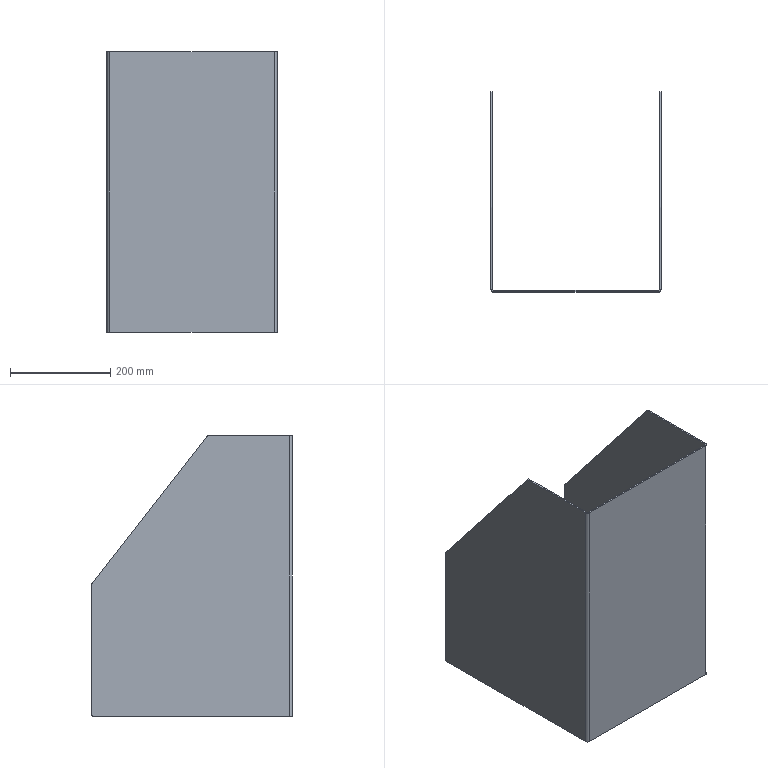Part | SolidWorks | features FlatPattern 1, ICE 1, SMBaseFlange 1, SheetMetal 1 | 1 solid | 30 faces | box 340 x 401 x 560 mm | volume 1696570 mm3 | plane 20 | cylinder 10 | commonest cylinder face diameters 6 x8 12 x2
STEP:
#1=CARTESIAN_POINT('',(340.,398.,0.));
#2=VERTEX_POINT('',#1);
#3=CARTESIAN_POINT('',(340.,401.,3.));
#4=VERTEX_POINT('',#3);
#5=CARTESIAN_POINT('',(340.,398.,3.));
#6=DIRECTION('',(1.,0.,0.));
#7=DIRECTION('',(0.,0.,1.));
#8=AXIS2_PLACEMENT_3D('',#5,#6,#7);
#9=CIRCLE('',#8,3.);
#10=EDGE_CURVE('',#2,#4,#9,.T.);
#11=ORIENTED_EDGE('',*,*,#10,.T.);
#12=CARTESIAN_POINT('',(340.,401.,262.937));
#13=VERTEX_POINT('',#12);
#14=CARTESIAN_POINT('',(340.,401.,560.));
#15=DIRECTION('',(0.,0.,-1.));
#16=VECTOR('',#15,1000.);
#17=LINE('',#14,#16);
#18=EDGE_CURVE('',#13,#4,#17,.T.);
#19=ORIENTED_EDGE('',*,*,#18,.F.);
#20=CARTESIAN_POINT('',(340.,400.364,264.784));
#21=VERTEX_POINT('',#20);
#22=CARTESIAN_POINT('',(340.,398.,262.937));
#23=DIRECTION('',(1.,0.,0.));
#24=DIRECTION('',(0.,0.,1.));
#25=AXIS2_PLACEMENT_3D('',#22,#23,#24);
#26=CIRCLE('',#25,3.);
#27=EDGE_CURVE('',#13,#21,#26,.T.);
#28=ORIENTED_EDGE('',*,*,#27,.T.);
#29=CARTESIAN_POINT('',(340.,170.611,558.847));
#30=VERTEX_POINT('',#29);
#31=CARTESIAN_POINT('',(340.,105.381,642.335));
#32=DIRECTION('',(0.,-0.6157,0.788));
#33=VECTOR('',#32,1000.);
#34=LINE('',#31,#33);
#35=EDGE_CURVE('',#21,#30,#34,.T.);
#36=ORIENTED_EDGE('',*,*,#35,.T.);
#37=CARTESIAN_POINT('',(340.,168.247,560.));
#38=VERTEX_POINT('',#37);
#39=CARTESIAN_POINT('',(340.,168.247,557.));
#40=DIRECTION('',(1.,0.,0.));
#41=DIRECTION('',(0.,0.,1.));
#42=AXIS2_PLACEMENT_3D('',#39,#40,#41);
#43=CIRCLE('',#42,3.);
#44=EDGE_CURVE('',#30,#38,#43,.T.);
#45=ORIENTED_EDGE('',*,*,#44,.T.);
#46=CARTESIAN_POINT('',(340.,6.,560.));
#47=VERTEX_POINT('',#46);
#48=CARTESIAN_POINT('',(340.,0.,560.));
#49=DIRECTION('',(0.,1.,0.));
#50=VECTOR('',#49,1000.);
#51=LINE('',#48,#50);
#52=EDGE_CURVE('',#47,#38,#51,.T.);
#53=ORIENTED_EDGE('',*,*,#52,.F.);
#54=CARTESIAN_POINT('',(340.,6.,0.));
#55=VERTEX_POINT('',#54);
#56=CARTESIAN_POINT('',(340.,6.,560.));
#57=DIRECTION('',(0.,0.,-1.));
#58=VECTOR('',#57,1000.);
#59=LINE('',#56,#58);
#60=EDGE_CURVE('',#47,#55,#59,.T.);
#61=ORIENTED_EDGE('',*,*,#60,.T.);
#62=CARTESIAN_POINT('',(340.,0.,0.));
#63=DIRECTION('',(0.,1.,0.));
#64=VECTOR('',#63,1000.);
#65=LINE('',#62,#64);
#66=EDGE_CURVE('',#55,#2,#65,.T.);
#67=ORIENTED_EDGE('',*,*,#66,.T.);
#68=EDGE_LOOP('',(#11,#19,#28,#36,#45,#53,#61,#67));
#69=FACE_OUTER_BOUND('',#68,.T.);
#70=CARTESIAN_POINT('',(340.,0.,560.));
#71=DIRECTION('',(-1.,0.,0.));
#72=DIRECTION('',(0.,0.,1.));
#73=AXIS2_PLACEMENT_3D('',#70,#71,#72);
#74=PLANE('',#73);
#75=ADVANCED_FACE('',(#69),#74,.F.);
#76=CARTESIAN_POINT('',(337.,401.,262.937));
#77=VERTEX_POINT('',#76);
#78=CARTESIAN_POINT('',(337.,401.,3.));
#79=VERTEX_POINT('',#78);
#80=CARTESIAN_POINT('',(337.,401.,560.));
#81=DIRECTION('',(0.,0.,-1.));
#82=VECTOR('',#81,1000.);
#83=LINE('',#80,#82);
#84=EDGE_CURVE('',#77,#79,#83,.T.);
#85=ORIENTED_EDGE('',*,*,#84,.T.);
#86=CARTESIAN_POINT('',(337.,398.,0.));
#87=VERTEX_POINT('',#86);
#88=CARTESIAN_POINT('',(337.,398.,3.));
#89=DIRECTION('',(1.,0.,0.));
#90=DIRECTION('',(0.,0.,1.));
#91=AXIS2_PLACEMENT_3D('',#88,#89,#90);
#92=CIRCLE('',#91,3.);
#93=EDGE_CURVE('',#87,#79,#92,.T.);
#94=ORIENTED_EDGE('',*,*,#93,.F.);
#95=CARTESIAN_POINT('',(337.,6.,0.));
#96=VERTEX_POINT('',#95);
#97=CARTESIAN_POINT('',(337.,0.,0.));
#98=DIRECTION('',(0.,1.,0.));
#99=VECTOR('',#98,1000.);
#100=LINE('',#97,#99);
#101=EDGE_CURVE('',#96,#87,#100,.T.);
#102=ORIENTED_EDGE('',*,*,#101,.F.);
#103=CARTESIAN_POINT('',(337.,6.,560.));
#104=VERTEX_POINT('',#103);
#105=CARTESIAN_POINT('',(337.,6.,560.));
#106=DIRECTION('',(0.,0.,-1.));
#107=VECTOR('',#106,1000.);
#108=LINE('',#105,#107);
#109=EDGE_CURVE('',#104,#96,#108,.T.);
#110=ORIENTED_EDGE('',*,*,#109,.F.);
#111=CARTESIAN_POINT('',(337.,168.247,560.));
#112=VERTEX_POINT('',#111);
#113=CARTESIAN_POINT('',(337.,0.,560.));
#114=DIRECTION('',(0.,1.,0.));
#115=VECTOR('',#114,1000.);
#116=LINE('',#113,#115);
#117=EDGE_CURVE('',#104,#112,#116,.T.);
#118=ORIENTED_EDGE('',*,*,#117,.T.);
#119=CARTESIAN_POINT('',(337.,170.611,558.847));
#120=VERTEX_POINT('',#119);
#121=CARTESIAN_POINT('',(337.,168.247,557.));
#122=DIRECTION('',(1.,0.,0.));
#123=DIRECTION('',(0.,0.,1.));
#124=AXIS2_PLACEMENT_3D('',#121,#122,#123);
#125=CIRCLE('',#124,3.);
#126=EDGE_CURVE('',#120,#112,#125,.T.);
#127=ORIENTED_EDGE('',*,*,#126,.F.);
#128=CARTESIAN_POINT('',(337.,400.364,264.784));
#129=VERTEX_POINT('',#128);
#130=CARTESIAN_POINT('',(337.,105.381,642.335));
#131=DIRECTION('',(0.,-0.6157,0.788));
#132=VECTOR('',#131,1000.);
#133=LINE('',#130,#132);
#134=EDGE_CURVE('',#129,#120,#133,.T.);
#135=ORIENTED_EDGE('',*,*,#134,.F.);
#136=CARTESIAN_POINT('',(337.,398.,262.937));
#137=DIRECTION('',(1.,0.,0.));
#138=DIRECTION('',(0.,0.,1.));
#139=AXIS2_PLACEMENT_3D('',#136,#137,#138);
#140=CIRCLE('',#139,3.);
#141=EDGE_CURVE('',#77,#129,#140,.T.);
#142=ORIENTED_EDGE('',*,*,#141,.F.);
#143=EDGE_LOOP('',(#85,#94,#102,#110,#118,#127,#135,#142));
#144=FACE_OUTER_BOUND('',#143,.T.);
#145=CARTESIAN_POINT('',(337.,0.,560.));
#146=DIRECTION('',(-1.,0.,0.));
#147=DIRECTION('',(0.,0.,1.));
#148=AXIS2_PLACEMENT_3D('',#145,#146,#147);
#149=PLANE('',#148);
#150=ADVANCED_FACE('',(#144),#149,.T.);
#151=ORIENTED_EDGE('',*,*,#18,.T.);
#152=CARTESIAN_POINT('',(337.,401.,3.));
#153=DIRECTION('',(1.,0.,0.));
#154=VECTOR('',#153,1000.);
#155=LINE('',#152,#154);
#156=EDGE_CURVE('',#79,#4,#155,.T.);
#157=ORIENTED_EDGE('',*,*,#156,.F.);
#158=ORIENTED_EDGE('',*,*,#84,.F.);
#159=CARTESIAN_POINT('',(337.,401.,262.937));
#160=DIRECTION('',(1.,0.,0.));
#161=VECTOR('',#160,1000.);
#162=LINE('',#159,#161);
#163=EDGE_CURVE('',#77,#13,#162,.T.);
#164=ORIENTED_EDGE('',*,*,#163,.T.);
#165=EDGE_LOOP('',(#151,#157,#158,#164));
#166=FACE_OUTER_BOUND('',#165,.T.);
#167=CARTESIAN_POINT('',(337.,401.,560.));
#168=DIRECTION('',(0.,1.,0.));
#169=DIRECTION('',(0.,0.,1.));
#170=AXIS2_PLACEMENT_3D('',#167,#168,#169);
#171=PLANE('',#170);
#172=ADVANCED_FACE('',(#166),#171,.T.);
#173=CARTESIAN_POINT('',(3.,398.,0.));
#174=VERTEX_POINT('',#173);
#175=CARTESIAN_POINT('',(3.,6.,0.));
#176=VERTEX_POINT('',#175);
#177=CARTESIAN_POINT('',(3.,0.,0.));
#178=DIRECTION('',(0.,-1.,0.));
#179=VECTOR('',#178,1000.);
#180=LINE('',#177,#179);
#181=EDGE_CURVE('',#174,#176,#180,.T.);
#182=ORIENTED_EDGE('',*,*,#181,.F.);
#183=CARTESIAN_POINT('',(3.,401.,3.));
#184=VERTEX_POINT('',#183);
#185=CARTESIAN_POINT('',(3.,398.,3.));
#186=DIRECTION('',(-1.,0.,0.));
#187=DIRECTION('',(0.,0.,-1.));
#188=AXIS2_PLACEMENT_3D('',#185,#186,#187);
#189=CIRCLE('',#188,3.);
#190=EDGE_CURVE('',#184,#174,#189,.T.);
#191=ORIENTED_EDGE('',*,*,#190,.F.);
#192=CARTESIAN_POINT('',(3.,401.,262.937));
#193=VERTEX_POINT('',#192);
#194=CARTESIAN_POINT('',(3.,401.,560.));
#195=DIRECTION('',(0.,0.,-1.));
#196=VECTOR('',#195,1000.);
#197=LINE('',#194,#196);
#198=EDGE_CURVE('',#193,#184,#197,.T.);
#199=ORIENTED_EDGE('',*,*,#198,.F.);
#200=CARTESIAN_POINT('',(3.,400.364,264.784));
#201=VERTEX_POINT('',#200);
#202=CARTESIAN_POINT('',(3.,398.,262.937));
#203=DIRECTION('',(-1.,0.,0.));
#204=DIRECTION('',(0.,0.,-1.));
#205=AXIS2_PLACEMENT_3D('',#202,#203,#204);
#206=CIRCLE('',#205,3.);
#207=EDGE_CURVE('',#201,#193,#206,.T.);
#208=ORIENTED_EDGE('',*,*,#207,.F.);
#209=CARTESIAN_POINT('',(3.,170.611,558.847));
#210=VERTEX_POINT('',#209);
#211=CARTESIAN_POINT('',(3.,105.381,642.335));
#212=DIRECTION('',(0.,0.6157,-0.788));
#213=VECTOR('',#212,1000.);
#214=LINE('',#211,#213);
#215=EDGE_CURVE('',#210,#201,#214,.T.);
#216=ORIENTED_EDGE('',*,*,#215,.F.);
#217=CARTESIAN_POINT('',(3.,168.247,560.));
#218=VERTEX_POINT('',#217);
#219=CARTESIAN_POINT('',(3.,168.247,557.));
#220=DIRECTION('',(-1.,0.,0.));
#221=DIRECTION('',(0.,0.,-1.));
#222=AXIS2_PLACEMENT_3D('',#219,#220,#221);
#223=CIRCLE('',#222,3.);
#224=EDGE_CURVE('',#218,#210,#223,.T.);
#225=ORIENTED_EDGE('',*,*,#224,.F.);
#226=CARTESIAN_POINT('',(3.,6.,560.));
#227=VERTEX_POINT('',#226);
#228=CARTESIAN_POINT('',(3.,0.,560.));
#229=DIRECTION('',(0.,-1.,0.));
#230=VECTOR('',#229,1000.);
#231=LINE('',#228,#230);
#232=EDGE_CURVE('',#218,#227,#231,.T.);
#233=ORIENTED_EDGE('',*,*,#232,.T.);
#234=CARTESIAN_POINT('',(3.,6.,560.));
#235=DIRECTION('',(0.,0.,-1.));
#236=VECTOR('',#235,1000.);
#237=LINE('',#234,#236);
#238=EDGE_CURVE('',#227,#176,#237,.T.);
#239=ORIENTED_EDGE('',*,*,#238,.T.);
#240=EDGE_LOOP('',(#182,#191,#199,#208,#216,#225,#233,#239));
#241=FACE_OUTER_BOUND('',#240,.T.);
#242=CARTESIAN_POINT('',(3.,0.,560.));
#243=DIRECTION('',(1.,0.,0.));
#244=DIRECTION('',(0.,0.,-1.));
#245=AXIS2_PLACEMENT_3D('',#242,#243,#244);
#246=PLANE('',#245);
#247=ADVANCED_FACE('',(#241),#246,.T.);
#248=CARTESIAN_POINT('',(0.,401.,3.));
#249=VERTEX_POINT('',#248);
#250=CARTESIAN_POINT('',(0.,398.,0.));
#251=VERTEX_POINT('',#250);
#252=CARTESIAN_POINT('',(0.,398.,3.));
#253=DIRECTION('',(-1.,0.,0.));
#254=DIRECTION('',(0.,0.,-1.));
#255=AXIS2_PLACEMENT_3D('',#252,#253,#254);
#256=CIRCLE('',#255,3.);
#257=EDGE_CURVE('',#249,#251,#256,.T.);
#258=ORIENTED_EDGE('',*,*,#257,.T.);
#259=CARTESIAN_POINT('',(0.,6.,0.));
#260=VERTEX_POINT('',#259);
#261=CARTESIAN_POINT('',(0.,0.,0.));
#262=DIRECTION('',(0.,-1.,0.));
#263=VECTOR('',#262,1000.);
#264=LINE('',#261,#263);
#265=EDGE_CURVE('',#251,#260,#264,.T.);
#266=ORIENTED_EDGE('',*,*,#265,.T.);
#267=CARTESIAN_POINT('',(0.,6.,560.));
#268=VERTEX_POINT('',#267);
#269=CARTESIAN_POINT('',(0.,6.,560.));
#270=DIRECTION('',(0.,0.,-1.));
#271=VECTOR('',#270,1000.);
#272=LINE('',#269,#271);
#273=EDGE_CURVE('',#268,#260,#272,.T.);
#274=ORIENTED_EDGE('',*,*,#273,.F.);
#275=CARTESIAN_POINT('',(0.,168.247,560.));
#276=VERTEX_POINT('',#275);
#277=CARTESIAN_POINT('',(0.,0.,560.));
#278=DIRECTION('',(0.,-1.,0.));
#279=VECTOR('',#278,1000.);
#280=LINE('',#277,#279);
#281=EDGE_CURVE('',#276,#268,#280,.T.);
#282=ORIENTED_EDGE('',*,*,#281,.F.);
#283=CARTESIAN_POINT('',(0.,170.611,558.847));
#284=VERTEX_POINT('',#283);
#285=CARTESIAN_POINT('',(0.,168.247,557.));
#286=DIRECTION('',(-1.,0.,0.));
#287=DIRECTION('',(0.,0.,-1.));
#288=AXIS2_PLACEMENT_3D('',#285,#286,#287);
#289=CIRCLE('',#288,3.);
#290=EDGE_CURVE('',#276,#284,#289,.T.);
#291=ORIENTED_EDGE('',*,*,#290,.T.);
#292=CARTESIAN_POINT('',(0.,400.364,264.784));
#293=VERTEX_POINT('',#292);
#294=CARTESIAN_POINT('',(0.,105.381,642.335));
#295=DIRECTION('',(0.,0.6157,-0.788));
#296=VECTOR('',#295,1000.);
#297=LINE('',#294,#296);
#298=EDGE_CURVE('',#284,#293,#297,.T.);
#299=ORIENTED_EDGE('',*,*,#298,.T.);
#300=CARTESIAN_POINT('',(0.,401.,262.937));
#301=VERTEX_POINT('',#300);
#302=CARTESIAN_POINT('',(0.,398.,262.937));
#303=DIRECTION('',(-1.,0.,0.));
#304=DIRECTION('',(0.,0.,-1.));
#305=AXIS2_PLACEMENT_3D('',#302,#303,#304);
#306=CIRCLE('',#305,3.);
#307=EDGE_CURVE('',#293,#301,#306,.T.);
#308=ORIENTED_EDGE('',*,*,#307,.T.);
#309=CARTESIAN_POINT('',(0.,401.,560.));
#310=DIRECTION('',(0.,0.,-1.));
#311=VECTOR('',#310,1000.);
#312=LINE('',#309,#311);
#313=EDGE_CURVE('',#301,#249,#312,.T.);
#314=ORIENTED_EDGE('',*,*,#313,.T.);
#315=EDGE_LOOP('',(#258,#266,#274,#282,#291,#299,#308,#314));
#316=FACE_OUTER_BOUND('',#315,.T.);
#317=CARTESIAN_POINT('',(0.,0.,560.));
#318=DIRECTION('',(1.,0.,0.));
#319=DIRECTION('',(0.,0.,-1.));
#320=AXIS2_PLACEMENT_3D('',#317,#318,#319);
#321=PLANE('',#320);
#322=ADVANCED_FACE('',(#316),#321,.F.);
#323=ORIENTED_EDGE('',*,*,#52,.T.);
#324=CARTESIAN_POINT('',(337.,168.247,560.));
#325=DIRECTION('',(1.,0.,0.));
#326=VECTOR('',#325,1000.);
#327=LINE('',#324,#326);
#328=EDGE_CURVE('',#112,#38,#327,.T.);
#329=ORIENTED_EDGE('',*,*,#328,.F.);
#330=ORIENTED_EDGE('',*,*,#117,.F.);
#331=CARTESIAN_POINT('',(337.,6.,560.));
#332=DIRECTION('',(1.,0.,0.));
#333=VECTOR('',#332,1000.);
#334=LINE('',#331,#333);
#335=EDGE_CURVE('',#104,#47,#334,.T.);
#336=ORIENTED_EDGE('',*,*,#335,.T.);
#337=EDGE_LOOP('',(#323,#329,#330,#336));
#338=FACE_OUTER_BOUND('',#337,.T.);
#339=CARTESIAN_POINT('',(334.,6.,560.));
#340=DIRECTION('',(0.,0.,1.));
#341=DIRECTION('',(1.,0.,0.));
#342=AXIS2_PLACEMENT_3D('',#339,#340,#341);
#343=PLANE('',#342);
#344=ADVANCED_FACE('',(#338),#343,.T.);
#345=CARTESIAN_POINT('',(3.,401.,3.));
#346=DIRECTION('',(-1.,0.,0.));
#347=VECTOR('',#346,1000.);
#348=LINE('',#345,#347);
#349=EDGE_CURVE('',#184,#249,#348,.T.);
#350=ORIENTED_EDGE('',*,*,#349,.T.);
#351=ORIENTED_EDGE('',*,*,#313,.F.);
#352=CARTESIAN_POINT('',(3.,401.,262.937));
#353=DIRECTION('',(-1.,0.,0.));
#354=VECTOR('',#353,1000.);
#355=LINE('',#352,#354);
#356=EDGE_CURVE('',#193,#301,#355,.T.);
#357=ORIENTED_EDGE('',*,*,#356,.F.);
#358=ORIENTED_EDGE('',*,*,#198,.T.);
#359=EDGE_LOOP('',(#350,#351,#357,#358));
#360=FACE_OUTER_BOUND('',#359,.T.);
#361=CARTESIAN_POINT('',(0.,401.,560.));
#362=DIRECTION('',(0.,1.,0.));
#363=DIRECTION('',(0.,0.,1.));
#364=AXIS2_PLACEMENT_3D('',#361,#362,#363);
#365=PLANE('',#364);
#366=ADVANCED_FACE('',(#360),#365,.T.);
#367=CARTESIAN_POINT('',(0.,6.,560.));
#368=DIRECTION('',(1.,0.,0.));
#369=VECTOR('',#368,1000.);
#370=LINE('',#367,#369);
#371=EDGE_CURVE('',#268,#227,#370,.T.);
#372=ORIENTED_EDGE('',*,*,#371,.F.);
#373=CARTESIAN_POINT('',(6.,0.,560.));
#374=VERTEX_POINT('',#373);
#375=CARTESIAN_POINT('',(6.,6.,560.));
#376=DIRECTION('',(0.,0.,1.));
#377=DIRECTION('',(-1.,0.,0.));
#378=AXIS2_PLACEMENT_3D('',#375,#376,#377);
#379=CIRCLE('',#378,6.);
#380=EDGE_CURVE('',#268,#374,#379,.T.);
#381=ORIENTED_EDGE('',*,*,#380,.T.);
#382=CARTESIAN_POINT('',(6.,3.,560.));
#383=VERTEX_POINT('',#382);
#384=CARTESIAN_POINT('',(6.,3.,560.));
#385=DIRECTION('',(0.,-1.,0.));
#386=VECTOR('',#385,1000.);
#387=LINE('',#384,#386);
#388=EDGE_CURVE('',#383,#374,#387,.T.);
#389=ORIENTED_EDGE('',*,*,#388,.F.);
#390=CARTESIAN_POINT('',(6.,6.,560.));
#391=DIRECTION('',(0.,0.,1.));
#392=DIRECTION('',(1.,0.,0.));
#393=AXIS2_PLACEMENT_3D('',#390,#391,#392);
#394=CIRCLE('',#393,3.);
#395=EDGE_CURVE('',#227,#383,#394,.T.);
#396=ORIENTED_EDGE('',*,*,#395,.F.);
#397=EDGE_LOOP('',(#372,#381,#389,#396));
#398=FACE_OUTER_BOUND('',#397,.T.);
#399=CARTESIAN_POINT('',(0.,6.,560.));
#400=DIRECTION('',(0.,0.,1.));
#401=DIRECTION('',(1.,0.,0.));
#402=AXIS2_PLACEMENT_3D('',#399,#400,#401);
#403=PLANE('',#402);
#404=ADVANCED_FACE('',(#398),#403,.T.);
#405=CARTESIAN_POINT('',(3.,168.247,560.));
#406=DIRECTION('',(-1.,0.,0.));
#407=VECTOR('',#406,1000.);
#408=LINE('',#405,#407);
#409=EDGE_CURVE('',#218,#276,#408,.T.);
#410=ORIENTED_EDGE('',*,*,#409,.T.);
#411=ORIENTED_EDGE('',*,*,#281,.T.);
#412=ORIENTED_EDGE('',*,*,#371,.T.);
#413=ORIENTED_EDGE('',*,*,#232,.F.);
#414=EDGE_LOOP('',(#410,#411,#412,#413));
#415=FACE_OUTER_BOUND('',#414,.T.);
#416=CARTESIAN_POINT('',(6.,3.,560.));
#417=DIRECTION('',(0.,0.,1.));
#418=DIRECTION('',(1.,0.,0.));
#419=AXIS2_PLACEMENT_3D('',#416,#417,#418);
#420=PLANE('',#419);
#421=ADVANCED_FACE('',(#415),#420,.T.);
#422=CARTESIAN_POINT('',(6.,0.,0.));
#423=VERTEX_POINT('',#422);
#424=CARTESIAN_POINT('',(6.,3.,0.));
#425=VERTEX_POINT('',#424);
#426=CARTESIAN_POINT('',(6.,0.,0.));
#427=DIRECTION('',(0.,1.,0.));
#428=VECTOR('',#427,1000.);
#429=LINE('',#426,#428);
#430=EDGE_CURVE('',#423,#425,#429,.T.);
#431=ORIENTED_EDGE('',*,*,#430,.F.);
#432=CARTESIAN_POINT('',(6.,6.,0.));
#433=DIRECTION('',(0.,0.,1.));
#434=DIRECTION('',(-1.,0.,0.));
#435=AXIS2_PLACEMENT_3D('',#432,#433,#434);
#436=CIRCLE('',#435,6.);
#437=EDGE_CURVE('',#260,#423,#436,.T.);
#438=ORIENTED_EDGE('',*,*,#437,.F.);
#439=CARTESIAN_POINT('',(3.,6.,0.));
#440=DIRECTION('',(-1.,0.,0.));
#441=VECTOR('',#440,1000.);
#442=LINE('',#439,#441);
#443=EDGE_CURVE('',#176,#260,#442,.T.);
#444=ORIENTED_EDGE('',*,*,#443,.F.);
#445=CARTESIAN_POINT('',(6.,6.,0.));
#446=DIRECTION('',(0.,0.,1.));
#447=DIRECTION('',(1.,0.,0.));
#448=AXIS2_PLACEMENT_3D('',#445,#446,#447);
#449=CIRCLE('',#448,3.);
#450=EDGE_CURVE('',#176,#425,#449,.T.);
#451=ORIENTED_EDGE('',*,*,#450,.T.);
#452=EDGE_LOOP('',(#431,#438,#444,#451));
#453=FACE_OUTER_BOUND('',#452,.T.);
#454=CARTESIAN_POINT('',(6.,0.,0.));
#455=DIRECTION('',(0.,0.,-1.));
#456=DIRECTION('',(-1.,0.,0.));
#457=AXIS2_PLACEMENT_3D('',#454,#455,#456);
#458=PLANE('',#457);
#459=ADVANCED_FACE('',(#453),#458,.T.);
#460=CARTESIAN_POINT('',(334.,0.,0.));
#461=VERTEX_POINT('',#460);
#462=CARTESIAN_POINT('',(0.,0.,0.));
#463=DIRECTION('',(1.,0.,0.));
#464=VECTOR('',#463,1000.);
#465=LINE('',#462,#464);
#466=EDGE_CURVE('',#423,#461,#465,.T.);
#467=ORIENTED_EDGE('',*,*,#466,.F.);
#468=ORIENTED_EDGE('',*,*,#430,.T.);
#469=CARTESIAN_POINT('',(334.,3.,0.));
#470=VERTEX_POINT('',#469);
#471=CARTESIAN_POINT('',(0.,3.,0.));
#472=DIRECTION('',(1.,0.,0.));
#473=VECTOR('',#472,1000.);
#474=LINE('',#471,#473);
#475=EDGE_CURVE('',#425,#470,#474,.T.);
#476=ORIENTED_EDGE('',*,*,#475,.T.);
#477=CARTESIAN_POINT('',(334.,3.,0.));
#478=DIRECTION('',(0.,-1.,0.));
#479=VECTOR('',#478,1000.);
#480=LINE('',#477,#479);
#481=EDGE_CURVE('',#470,#461,#480,.T.);
#482=ORIENTED_EDGE('',*,*,#481,.T.);
#483=EDGE_LOOP('',(#467,#468,#476,#482));
#484=FACE_OUTER_BOUND('',#483,.T.);
#485=CARTESIAN_POINT('',(3.,6.,0.));
#486=DIRECTION('',(0.,0.,-1.));
#487=DIRECTION('',(-1.,0.,0.));
#488=AXIS2_PLACEMENT_3D('',#485,#486,#487);
#489=PLANE('',#488);
#490=ADVANCED_FACE('',(#484),#489,.T.);
#491=CARTESIAN_POINT('',(334.,0.,560.));
#492=VERTEX_POINT('',#491);
#493=CARTESIAN_POINT('',(334.,3.,560.));
#494=VERTEX_POINT('',#493);
#495=CARTESIAN_POINT('',(334.,0.,560.));
#496=DIRECTION('',(0.,1.,0.));
#497=VECTOR('',#496,1000.);
#498=LINE('',#495,#497);
#499=EDGE_CURVE('',#492,#494,#498,.T.);
#500=ORIENTED_EDGE('',*,*,#499,.F.);
#501=CARTESIAN_POINT('',(334.,6.,560.));
#502=DIRECTION('',(0.,0.,1.));
#503=DIRECTION('',(-1.,0.,0.));
#504=AXIS2_PLACEMENT_3D('',#501,#502,#503);
#505=CIRCLE('',#504,6.);
#506=EDGE_CURVE('',#492,#47,#505,.T.);
#507=ORIENTED_EDGE('',*,*,#506,.T.);
#508=ORIENTED_EDGE('',*,*,#335,.F.);
#509=CARTESIAN_POINT('',(334.,6.,560.));
#510=DIRECTION('',(0.,0.,1.));
#511=DIRECTION('',(1.,0.,0.));
#512=AXIS2_PLACEMENT_3D('',#509,#510,#511);
#513=CIRCLE('',#512,3.);
#514=EDGE_CURVE('',#494,#104,#513,.T.);
#515=ORIENTED_EDGE('',*,*,#514,.F.);
#516=EDGE_LOOP('',(#500,#507,#508,#515));
#517=FACE_OUTER_BOUND('',#516,.T.);
#518=CARTESIAN_POINT('',(334.,0.,560.));
#519=DIRECTION('',(0.,0.,1.));
#520=DIRECTION('',(1.,0.,0.));
#521=AXIS2_PLACEMENT_3D('',#518,#519,#520);
#522=PLANE('',#521);
#523=ADVANCED_FACE('',(#517),#522,.T.);
#524=CARTESIAN_POINT('',(0.,0.,560.));
#525=DIRECTION('',(1.,0.,0.));
#526=VECTOR('',#525,1000.);
#527=LINE('',#524,#526);
#528=EDGE_CURVE('',#374,#492,#527,.T.);
#529=ORIENTED_EDGE('',*,*,#528,.T.);
#530=ORIENTED_EDGE('',*,*,#499,.T.);
#531=CARTESIAN_POINT('',(0.,3.,560.));
#532=DIRECTION('',(1.,0.,0.));
#533=VECTOR('',#532,1000.);
#534=LINE('',#531,#533);
#535=EDGE_CURVE('',#383,#494,#534,.T.);
#536=ORIENTED_EDGE('',*,*,#535,.F.);
#537=ORIENTED_EDGE('',*,*,#388,.T.);
#538=EDGE_LOOP('',(#529,#530,#536,#537));
#539=FACE_OUTER_BOUND('',#538,.T.);
#540=CARTESIAN_POINT('',(337.,6.,560.));
#541=DIRECTION('',(0.,0.,1.));
#542=DIRECTION('',(1.,0.,0.));
#543=AXIS2_PLACEMENT_3D('',#540,#541,#542);
#544=PLANE('',#543);
#545=ADVANCED_FACE('',(#539),#544,.T.);
#546=CARTESIAN_POINT('',(340.,6.,0.));
#547=DIRECTION('',(-1.,0.,0.));
#548=VECTOR('',#547,1000.);
#549=LINE('',#546,#548);
#550=EDGE_CURVE('',#55,#96,#549,.T.);
#551=ORIENTED_EDGE('',*,*,#550,.F.);
#552=CARTESIAN_POINT('',(334.,6.,0.));
#553=DIRECTION('',(0.,0.,1.));
#554=DIRECTION('',(-1.,0.,0.));
#555=AXIS2_PLACEMENT_3D('',#552,#553,#554);
#556=CIRCLE('',#555,6.);
#557=EDGE_CURVE('',#461,#55,#556,.T.);
#558=ORIENTED_EDGE('',*,*,#557,.F.);
#559=ORIENTED_EDGE('',*,*,#481,.F.);
#560=CARTESIAN_POINT('',(334.,6.,0.));
#561=DIRECTION('',(0.,0.,1.));
#562=DIRECTION('',(1.,0.,0.));
#563=AXIS2_PLACEMENT_3D('',#560,#561,#562);
#564=CIRCLE('',#563,3.);
#565=EDGE_CURVE('',#470,#96,#564,.T.);
#566=ORIENTED_EDGE('',*,*,#565,.T.);
#567=EDGE_LOOP('',(#551,#558,#559,#566));
#568=FACE_OUTER_BOUND('',#567,.T.);
#569=CARTESIAN_POINT('',(340.,6.,0.));
#570=DIRECTION('',(0.,0.,-1.));
#571=DIRECTION('',(-1.,0.,0.));
#572=AXIS2_PLACEMENT_3D('',#569,#570,#571);
#573=PLANE('',#572);
#574=ADVANCED_FACE('',(#568),#573,.T.);
#575=CARTESIAN_POINT('',(337.,398.,0.));
#576=DIRECTION('',(1.,0.,0.));
#577=VECTOR('',#576,1000.);
#578=LINE('',#575,#577);
#579=EDGE_CURVE('',#87,#2,#578,.T.);
#580=ORIENTED_EDGE('',*,*,#579,.T.);
#581=ORIENTED_EDGE('',*,*,#66,.F.);
#582=ORIENTED_EDGE('',*,*,#550,.T.);
#583=ORIENTED_EDGE('',*,*,#101,.T.);
#584=EDGE_LOOP('',(#580,#581,#582,#583));
#585=FACE_OUTER_BOUND('',#584,.T.);
#586=CARTESIAN_POINT('',(334.,3.,0.));
#587=DIRECTION('',(0.,0.,-1.));
#588=DIRECTION('',(-1.,0.,0.));
#589=AXIS2_PLACEMENT_3D('',#586,#587,#588);
#590=PLANE('',#589);
#591=ADVANCED_FACE('',(#585),#590,.T.);
#592=ORIENTED_EDGE('',*,*,#565,.F.);
#593=CARTESIAN_POINT('',(334.,3.,560.));
#594=DIRECTION('',(0.,0.,-1.));
#595=VECTOR('',#594,1000.);
#596=LINE('',#593,#595);
#597=EDGE_CURVE('',#494,#470,#596,.T.);
#598=ORIENTED_EDGE('',*,*,#597,.F.);
#599=ORIENTED_EDGE('',*,*,#514,.T.);
#600=ORIENTED_EDGE('',*,*,#109,.T.);
#601=EDGE_LOOP('',(#592,#598,#599,#600));
#602=FACE_OUTER_BOUND('',#601,.T.);
#603=CARTESIAN_POINT('',(334.,6.,560.));
#604=DIRECTION('',(0.,0.,-1.));
#605=DIRECTION('',(-1.,0.,0.));
#606=AXIS2_PLACEMENT_3D('',#603,#604,#605);
#607=CYLINDRICAL_SURFACE('',#606,3.);
#608=ADVANCED_FACE('',(#602),#607,.F.);
#609=ORIENTED_EDGE('',*,*,#475,.F.);
#610=CARTESIAN_POINT('',(6.,3.,560.));
#611=DIRECTION('',(0.,0.,-1.));
#612=VECTOR('',#611,1000.);
#613=LINE('',#610,#612);
#614=EDGE_CURVE('',#383,#425,#613,.T.);
#615=ORIENTED_EDGE('',*,*,#614,.F.);
#616=ORIENTED_EDGE('',*,*,#535,.T.);
#617=ORIENTED_EDGE('',*,*,#597,.T.);
#618=EDGE_LOOP('',(#609,#615,#616,#617));
#619=FACE_OUTER_BOUND('',#618,.T.);
#620=CARTESIAN_POINT('',(0.,3.,560.));
#621=DIRECTION('',(0.,1.,0.));
#622=DIRECTION('',(0.,0.,1.));
#623=AXIS2_PLACEMENT_3D('',#620,#621,#622);
#624=PLANE('',#623);
#625=ADVANCED_FACE('',(#619),#624,.T.);
#626=ORIENTED_EDGE('',*,*,#450,.F.);
#627=ORIENTED_EDGE('',*,*,#238,.F.);
#628=ORIENTED_EDGE('',*,*,#395,.T.);
#629=ORIENTED_EDGE('',*,*,#614,.T.);
#630=EDGE_LOOP('',(#626,#627,#628,#629));
#631=FACE_OUTER_BOUND('',#630,.T.);
#632=CARTESIAN_POINT('',(6.,6.,560.));
#633=DIRECTION('',(0.,0.,-1.));
#634=DIRECTION('',(-1.,0.,0.));
#635=AXIS2_PLACEMENT_3D('',#632,#633,#634);
#636=CYLINDRICAL_SURFACE('',#635,3.);
#637=ADVANCED_FACE('',(#631),#636,.F.);
#638=ORIENTED_EDGE('',*,*,#437,.T.);
#639=CARTESIAN_POINT('',(6.,0.,560.));
#640=DIRECTION('',(0.,0.,-1.));
#641=VECTOR('',#640,1000.);
#642=LINE('',#639,#641);
#643=EDGE_CURVE('',#374,#423,#642,.T.);
#644=ORIENTED_EDGE('',*,*,#643,.F.);
#645=ORIENTED_EDGE('',*,*,#380,.F.);
#646=ORIENTED_EDGE('',*,*,#273,.T.);
#647=EDGE_LOOP('',(#638,#644,#645,#646));
#648=FACE_OUTER_BOUND('',#647,.T.);
#649=CARTESIAN_POINT('',(6.,6.,560.));
#650=DIRECTION('',(0.,0.,-1.));
#651=DIRECTION('',(-1.,0.,0.));
#652=AXIS2_PLACEMENT_3D('',#649,#650,#651);
#653=CYLINDRICAL_SURFACE('',#652,6.);
#654=ADVANCED_FACE('',(#648),#653,.T.);
#655=ORIENTED_EDGE('',*,*,#466,.T.);
#656=CARTESIAN_POINT('',(334.,0.,560.));
#657=DIRECTION('',(0.,0.,-1.));
#658=VECTOR('',#657,1000.);
#659=LINE('',#656,#658);
#660=EDGE_CURVE('',#492,#461,#659,.T.);
#661=ORIENTED_EDGE('',*,*,#660,.F.);
#662=ORIENTED_EDGE('',*,*,#528,.F.);
#663=ORIENTED_EDGE('',*,*,#643,.T.);
#664=EDGE_LOOP('',(#655,#661,#662,#663));
#665=FACE_OUTER_BOUND('',#664,.T.);
#666=CARTESIAN_POINT('',(0.,0.,560.));
#667=DIRECTION('',(0.,1.,0.));
#668=DIRECTION('',(0.,0.,1.));
#669=AXIS2_PLACEMENT_3D('',#666,#667,#668);
#670=PLANE('',#669);
#671=ADVANCED_FACE('',(#665),#670,.F.);
#672=ORIENTED_EDGE('',*,*,#557,.T.);
#673=ORIENTED_EDGE('',*,*,#60,.F.);
#674=ORIENTED_EDGE('',*,*,#506,.F.);
#675=ORIENTED_EDGE('',*,*,#660,.T.);
#676=EDGE_LOOP('',(#672,#673,#674,#675));
#677=FACE_OUTER_BOUND('',#676,.T.);
#678=CARTESIAN_POINT('',(334.,6.,560.));
#679=DIRECTION('',(0.,0.,-1.));
#680=DIRECTION('',(-1.,0.,0.));
#681=AXIS2_PLACEMENT_3D('',#678,#679,#680);
#682=CYLINDRICAL_SURFACE('',#681,6.);
#683=ADVANCED_FACE('',(#677),#682,.T.);
#684=ORIENTED_EDGE('',*,*,#265,.F.);
#685=CARTESIAN_POINT('',(3.,398.,0.));
#686=DIRECTION('',(-1.,0.,0.));
#687=VECTOR('',#686,1000.);
#688=LINE('',#685,#687);
#689=EDGE_CURVE('',#174,#251,#688,.T.);
#690=ORIENTED_EDGE('',*,*,#689,.F.);
#691=ORIENTED_EDGE('',*,*,#181,.T.);
#692=ORIENTED_EDGE('',*,*,#443,.T.);
#693=EDGE_LOOP('',(#684,#690,#691,#692));
#694=FACE_OUTER_BOUND('',#693,.T.);
#695=CARTESIAN_POINT('',(334.,6.,0.));
#696=DIRECTION('',(0.,0.,1.));
#697=DIRECTION('',(1.,0.,0.));
#698=AXIS2_PLACEMENT_3D('',#695,#696,#697);
#699=PLANE('',#698);
#700=ADVANCED_FACE('',(#694),#699,.F.);
#701=ORIENTED_EDGE('',*,*,#409,.F.);
#702=ORIENTED_EDGE('',*,*,#224,.T.);
#703=CARTESIAN_POINT('',(3.,170.611,558.847));
#704=DIRECTION('',(-1.,0.,0.));
#705=VECTOR('',#704,1000.);
#706=LINE('',#703,#705);
#707=EDGE_CURVE('',#210,#284,#706,.T.);
#708=ORIENTED_EDGE('',*,*,#707,.T.);
#709=ORIENTED_EDGE('',*,*,#290,.F.);
#710=EDGE_LOOP('',(#701,#702,#708,#709));
#711=FACE_OUTER_BOUND('',#710,.T.);
#712=CARTESIAN_POINT('',(3.,168.247,557.));
#713=DIRECTION('',(1.,0.,0.));
#714=DIRECTION('',(0.,0.,-1.));
#715=AXIS2_PLACEMENT_3D('',#712,#713,#714);
#716=CYLINDRICAL_SURFACE('',#715,3.);
#717=ADVANCED_FACE('',(#711),#716,.T.);
#718=ORIENTED_EDGE('',*,*,#707,.F.);
#719=ORIENTED_EDGE('',*,*,#215,.T.);
#720=CARTESIAN_POINT('',(3.,400.364,264.784));
#721=DIRECTION('',(-1.,0.,0.));
#722=VECTOR('',#721,1000.);
#723=LINE('',#720,#722);
#724=EDGE_CURVE('',#201,#293,#723,.T.);
#725=ORIENTED_EDGE('',*,*,#724,.T.);
#726=ORIENTED_EDGE('',*,*,#298,.F.);
#727=EDGE_LOOP('',(#718,#719,#725,#726));
#728=FACE_OUTER_BOUND('',#727,.T.);
#729=CARTESIAN_POINT('',(3.,105.381,642.335));
#730=DIRECTION('',(0.,-0.788,-0.6157));
#731=DIRECTION('',(0.,0.6157,-0.788));
#732=AXIS2_PLACEMENT_3D('',#729,#730,#731);
#733=PLANE('',#732);
#734=ADVANCED_FACE('',(#728),#733,.F.);
#735=ORIENTED_EDGE('',*,*,#207,.T.);
#736=ORIENTED_EDGE('',*,*,#356,.T.);
#737=ORIENTED_EDGE('',*,*,#307,.F.);
#738=ORIENTED_EDGE('',*,*,#724,.F.);
#739=EDGE_LOOP('',(#735,#736,#737,#738));
#740=FACE_OUTER_BOUND('',#739,.T.);
#741=CARTESIAN_POINT('',(3.,398.,262.937));
#742=DIRECTION('',(1.,0.,0.));
#743=DIRECTION('',(0.,0.,-1.));
#744=AXIS2_PLACEMENT_3D('',#741,#742,#743);
#745=CYLINDRICAL_SURFACE('',#744,3.);
#746=ADVANCED_FACE('',(#740),#745,.T.);
#747=ORIENTED_EDGE('',*,*,#163,.F.);
#748=ORIENTED_EDGE('',*,*,#141,.T.);
#749=CARTESIAN_POINT('',(337.,400.364,264.784));
#750=DIRECTION('',(1.,0.,0.));
#751=VECTOR('',#750,1000.);
#752=LINE('',#749,#751);
#753=EDGE_CURVE('',#129,#21,#752,.T.);
#754=ORIENTED_EDGE('',*,*,#753,.T.);
#755=ORIENTED_EDGE('',*,*,#27,.F.);
#756=EDGE_LOOP('',(#747,#748,#754,#755));
#757=FACE_OUTER_BOUND('',#756,.T.);
#758=CARTESIAN_POINT('',(337.,398.,262.937));
#759=DIRECTION('',(-1.,0.,0.));
#760=DIRECTION('',(0.,0.,1.));
#761=AXIS2_PLACEMENT_3D('',#758,#759,#760);
#762=CYLINDRICAL_SURFACE('',#761,3.);
#763=ADVANCED_FACE('',(#757),#762,.T.);
#764=ORIENTED_EDGE('',*,*,#753,.F.);
#765=ORIENTED_EDGE('',*,*,#134,.T.);
#766=CARTESIAN_POINT('',(337.,170.611,558.847));
#767=DIRECTION('',(1.,0.,0.));
#768=VECTOR('',#767,1000.);
#769=LINE('',#766,#768);
#770=EDGE_CURVE('',#120,#30,#769,.T.);
#771=ORIENTED_EDGE('',*,*,#770,.T.);
#772=ORIENTED_EDGE('',*,*,#35,.F.);
#773=EDGE_LOOP('',(#764,#765,#771,#772));
#774=FACE_OUTER_BOUND('',#773,.T.);
#775=CARTESIAN_POINT('',(337.,105.381,642.335));
#776=DIRECTION('',(0.,-0.788,-0.6157));
#777=DIRECTION('',(0.,-0.6157,0.788));
#778=AXIS2_PLACEMENT_3D('',#775,#776,#777);
#779=PLANE('',#778);
#780=ADVANCED_FACE('',(#774),#779,.F.);
#781=ORIENTED_EDGE('',*,*,#126,.T.);
#782=ORIENTED_EDGE('',*,*,#328,.T.);
#783=ORIENTED_EDGE('',*,*,#44,.F.);
#784=ORIENTED_EDGE('',*,*,#770,.F.);
#785=EDGE_LOOP('',(#781,#782,#783,#784));
#786=FACE_OUTER_BOUND('',#785,.T.);
#787=CARTESIAN_POINT('',(337.,168.247,557.));
#788=DIRECTION('',(-1.,0.,0.));
#789=DIRECTION('',(0.,0.,1.));
#790=AXIS2_PLACEMENT_3D('',#787,#788,#789);
#791=CYLINDRICAL_SURFACE('',#790,3.);
#792=ADVANCED_FACE('',(#786),#791,.T.);
#793=ORIENTED_EDGE('',*,*,#190,.T.);
#794=ORIENTED_EDGE('',*,*,#689,.T.);
#795=ORIENTED_EDGE('',*,*,#257,.F.);
#796=ORIENTED_EDGE('',*,*,#349,.F.);
#797=EDGE_LOOP('',(#793,#794,#795,#796));
#798=FACE_OUTER_BOUND('',#797,.T.);
#799=CARTESIAN_POINT('',(3.,398.,3.));
#800=DIRECTION('',(1.,0.,0.));
#801=DIRECTION('',(0.,0.,-1.));
#802=AXIS2_PLACEMENT_3D('',#799,#800,#801);
#803=CYLINDRICAL_SURFACE('',#802,3.);
#804=ADVANCED_FACE('',(#798),#803,.T.);
#805=ORIENTED_EDGE('',*,*,#93,.T.);
#806=ORIENTED_EDGE('',*,*,#156,.T.);
#807=ORIENTED_EDGE('',*,*,#10,.F.);
#808=ORIENTED_EDGE('',*,*,#579,.F.);
#809=EDGE_LOOP('',(#805,#806,#807,#808));
#810=FACE_OUTER_BOUND('',#809,.T.);
#811=CARTESIAN_POINT('',(337.,398.,3.));
#812=DIRECTION('',(-1.,0.,0.));
#813=DIRECTION('',(0.,0.,1.));
#814=AXIS2_PLACEMENT_3D('',#811,#812,#813);
#815=CYLINDRICAL_SURFACE('',#814,3.);
#816=ADVANCED_FACE('',(#810),#815,.T.);
#817=CLOSED_SHELL('',(#75,#150,#172,#247,#322,#344,#366,#404,#421,#459,#490,#523,#545,#574,#591,#608,#625,#637,#654,#671,#683,#700,#717,#734,#746,#763,#780,#792,#804,#816));
#818=MANIFOLD_SOLID_BREP('',#817);
#819=CARTESIAN_POINT('',(0.,0.,0.));
#820=DIRECTION('',(0.,0.,1.));
#821=DIRECTION('',(1.,0.,0.));
#822=AXIS2_PLACEMENT_3D('',#819,#820,#821);
#823=(LENGTH_UNIT()NAMED_UNIT(*)SI_UNIT(.MILLI.,.METRE.));
#824=UNCERTAINTY_MEASURE_WITH_UNIT(LENGTH_MEASURE(0.00001),#823,'','');
#825=(NAMED_UNIT(*)PLANE_ANGLE_UNIT()SI_UNIT($,.RADIAN.));
#826=(NAMED_UNIT(*)SI_UNIT($,.STERADIAN.)SOLID_ANGLE_UNIT());
#827=(GEOMETRIC_REPRESENTATION_CONTEXT(3)GLOBAL_UNCERTAINTY_ASSIGNED_CONTEXT((#824))GLOBAL_UNIT_ASSIGNED_CONTEXT((#823,#825,#826))REPRESENTATION_CONTEXT('',''));
#828=ADVANCED_BREP_SHAPE_REPRESENTATION('',(#818,#822),#827);